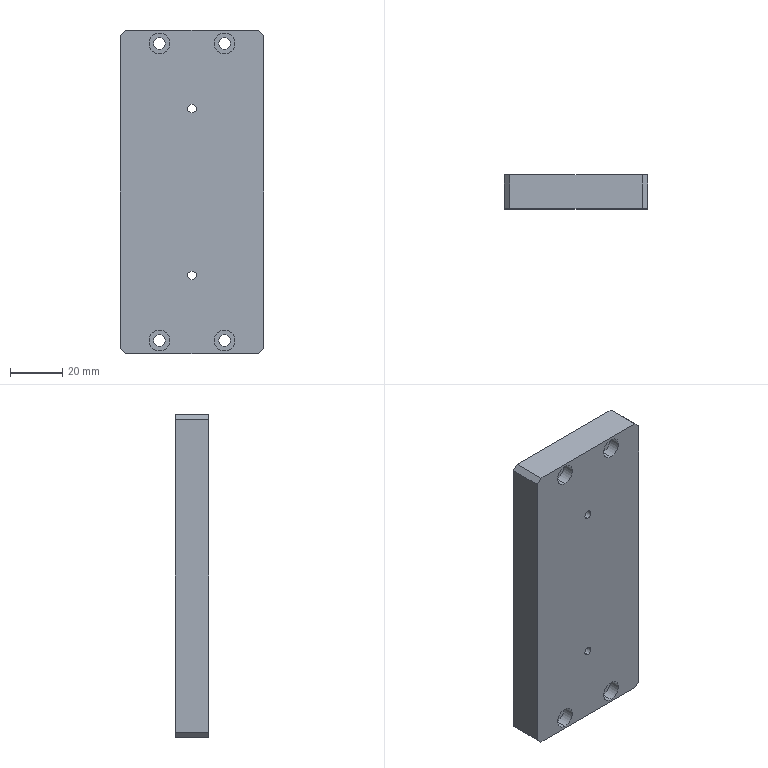Part | STEP file | (PA01.001.LX018) Idler Connecting Plate | 1 solid | 34 faces | box 55 x 13 x 124 mm | volume 86902 mm3 | cylinder 20 | plane 14 | commonest cylinder face diameters 4.5 x8 8 x8 3.3 x4